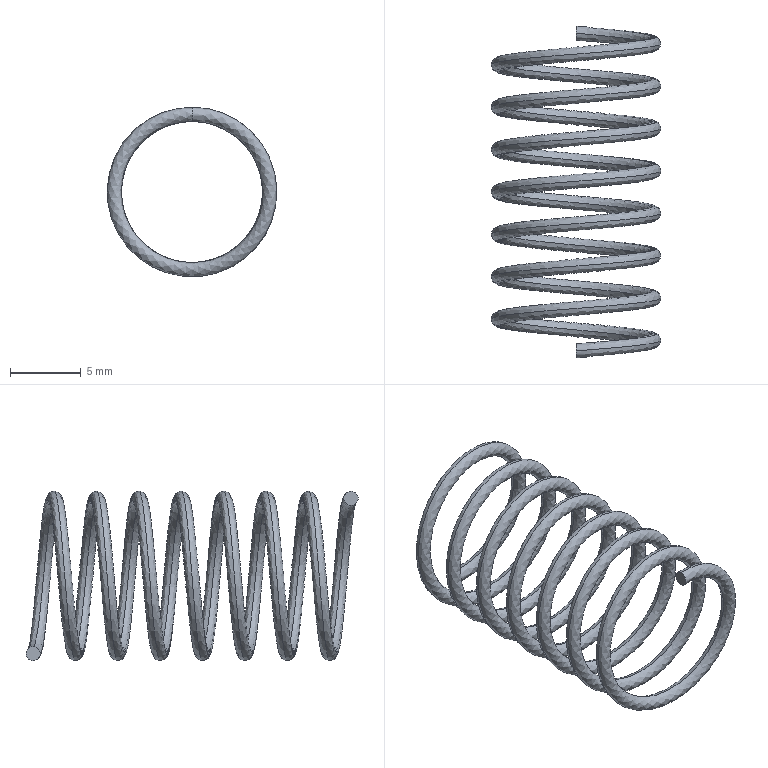Part | SolidWorks | features Helix 1, Sweep 1 | 1 solid | 4 faces | box 12 x 23.5 x 12 mm | volume 203.726 mm3 | spline 2 | plane 2